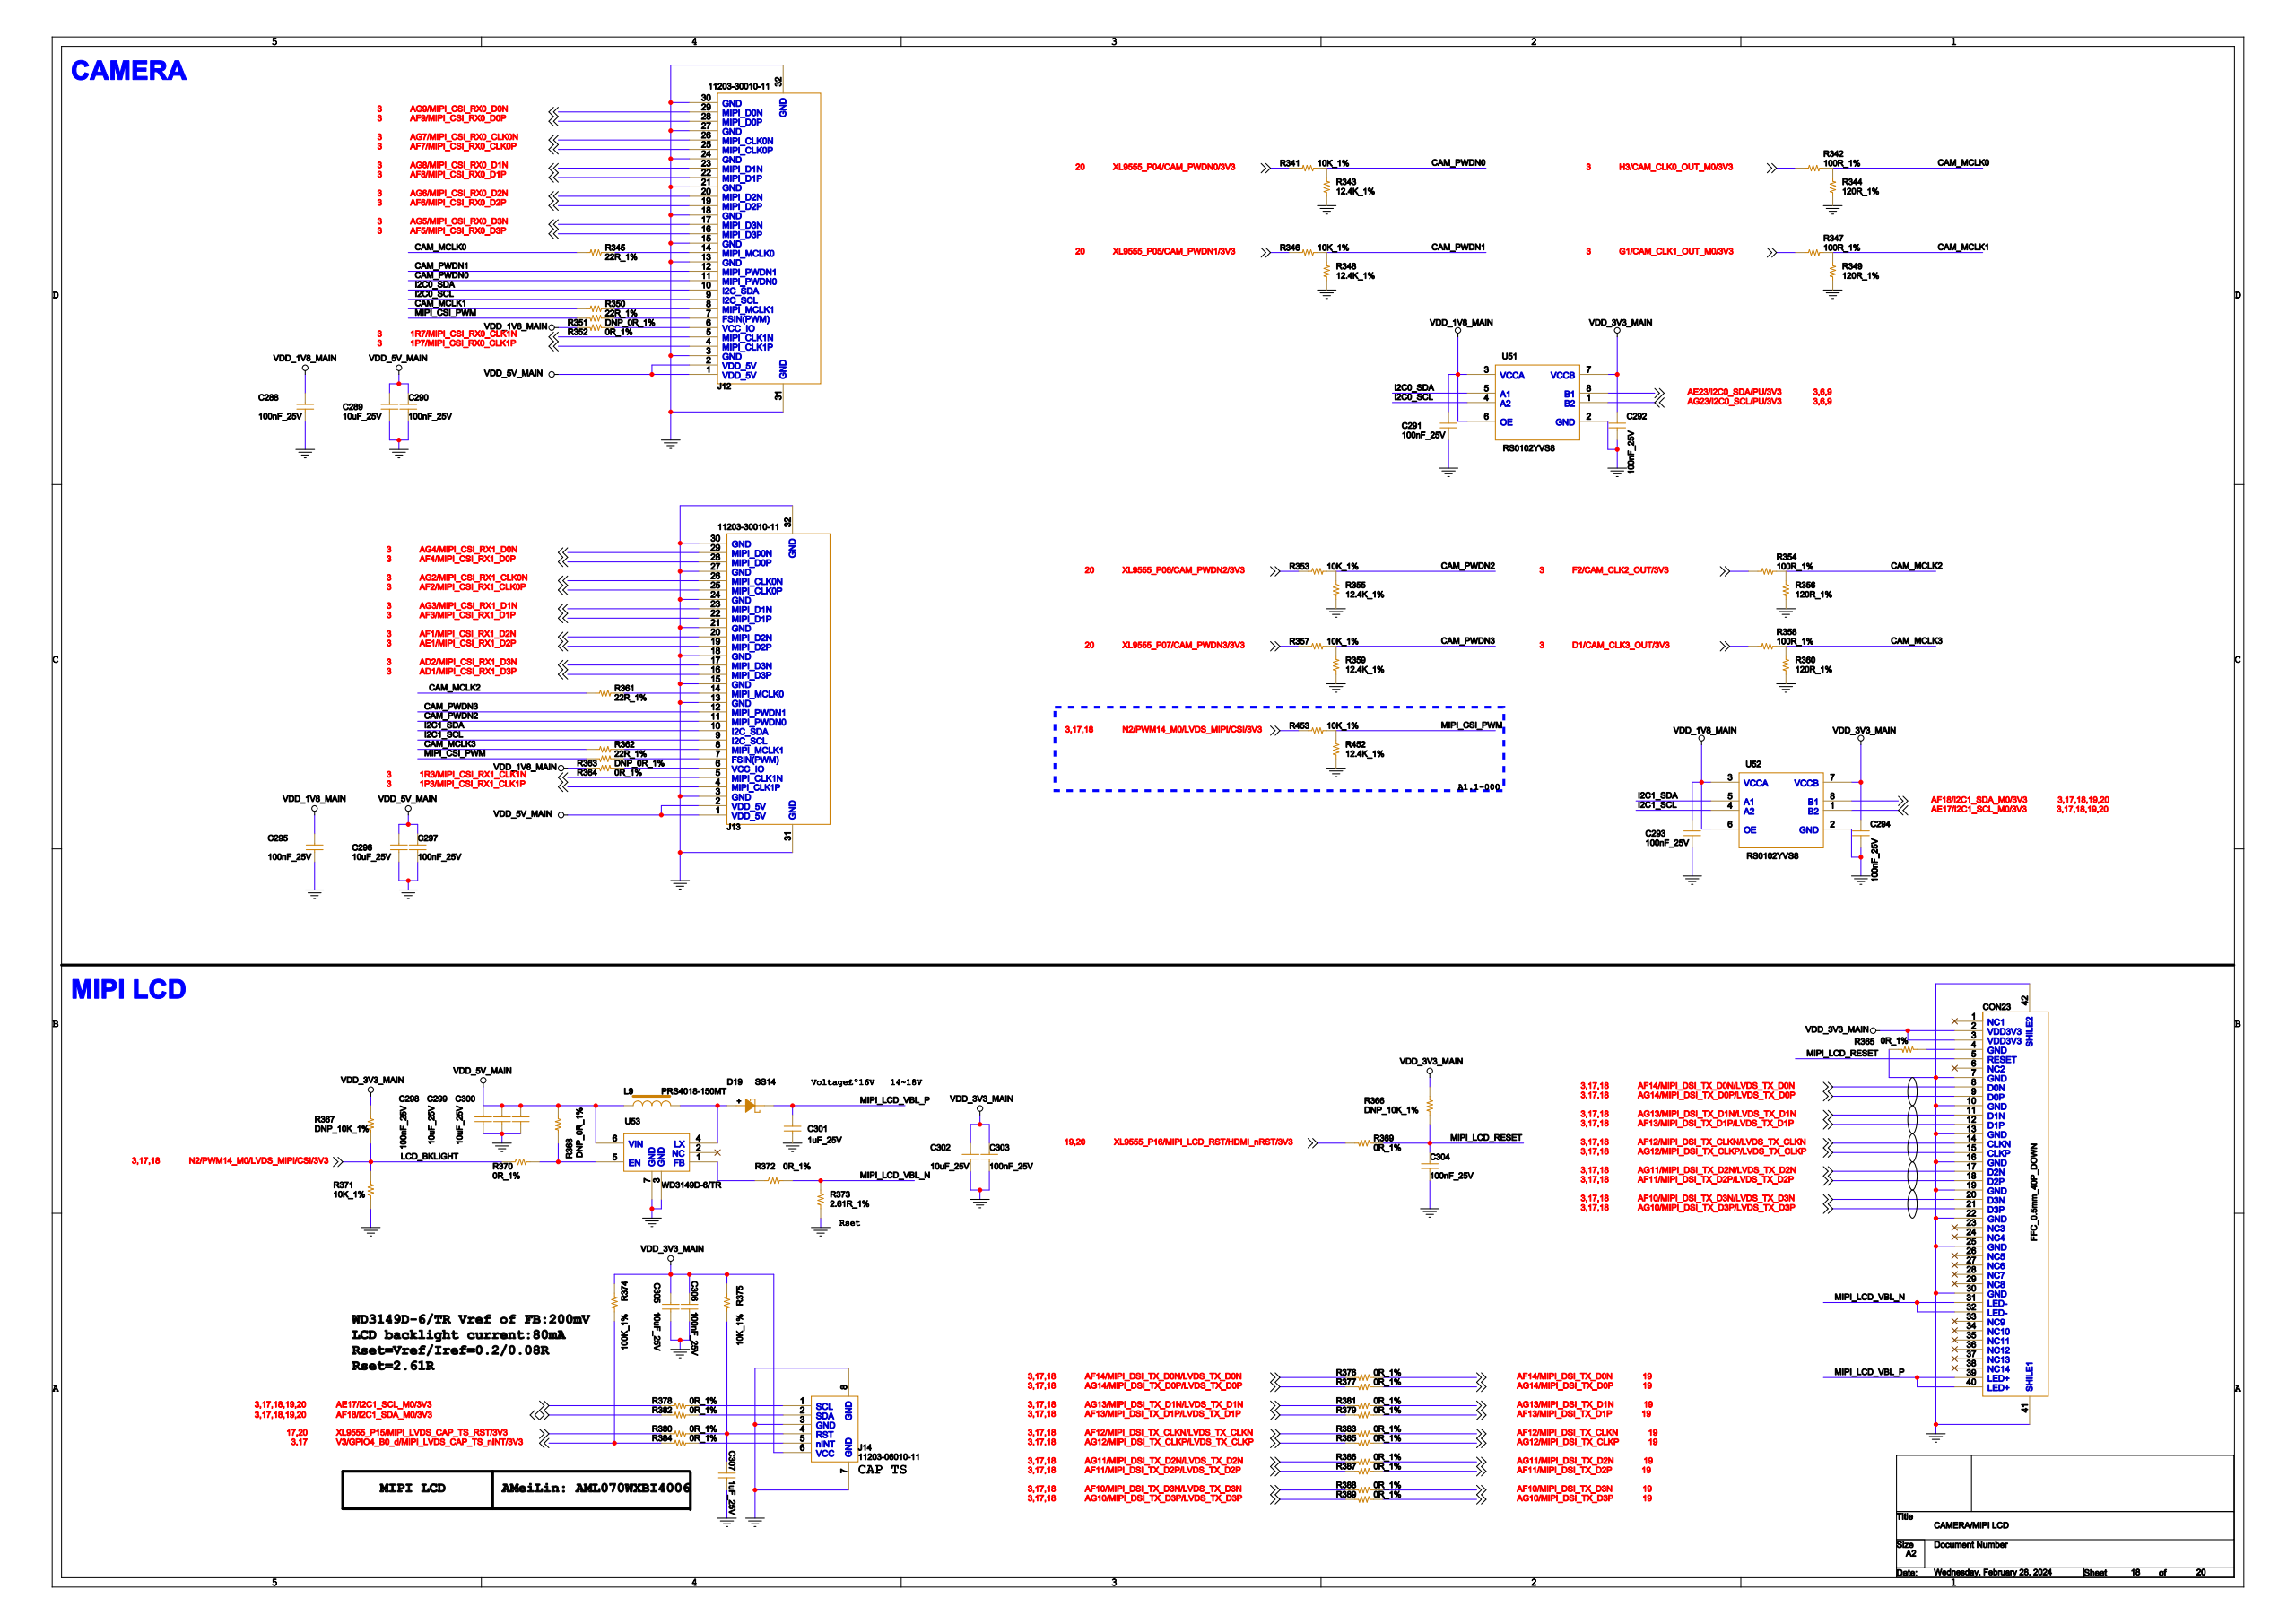Circuit board | Cadence Allegro | 1024 parts | 682 nets | one sheet of the schematic
Parts on this sheet (reference | value | footprint):
C288 | 100nF_25V | C0402
C289 | 10uF_25V | C0603
C290 | 100nF_25V | C0402
C291 | 100nF_25V | C0402
C292 | 100nF_25V | C0402
C293 | 100nF_25V | C0402
C294 | 100nF_25V | C0402
C295 | 100nF_25V | C0402
C296 | 10uF_25V | C0603
C297 | 100nF_25V | C0402
C298 | 100nF_25V | C0402
C299 | 10uF_25V | C0603
C300 | 10uF_25V | C0603
C301 | 1uF_25V | C0603
C302 | 10uF_25V | C0603
C303 | 100nF_25V | C0402
C304 | 100nF_25V | C0402
C305 | 10uF_25V | C0603
C306 | 100nF_25V | C0402
C307 | 1uF_25V | C0603
CON23 | FFC_0.5mm_40P_DOWN | CON_FFC_0D5_40P
D19 | SS14 | SMA
J12 | 11203-30010-11 | CON_FFC_0D5_30P
J13 | 11203-30010-11 | CON_FFC_0D5_30P
J14 | 11203-06010-11 | CON_FFC_0D5_6P
L9 | PRS4018-150MT | L_L4D5XW4D0_H3D2
R341 | 10K_1% | R0402
R342 | 100R_1% | R0603
R343 | 12.4K_1% | R0402
R344 | 120R_1% | R0603
R345 | 22R_1% | R0402
R346 | 10K_1% | R0402
R347 | 100R_1% | R0603
R348 | 12.4K_1% | R0402
R349 | 120R_1% | R0603
R350 | 22R_1% | R0402
R351 | DNP_0R_1% | R0402
R352 | 0R_1% | R0402
R353 | 10K_1% | R0402
R354 | 100R_1% | R0603
R355 | 12.4K_1% | R0402
R356 | 120R_1% | R0603
R357 | 10K_1% | R0402
R358 | 100R_1% | R0603
R359 | 12.4K_1% | R0402
R360 | 120R_1% | R0603
R361 | 22R_1% | R0402
R362 | 22R_1% | R0402
R363 | DNP_0R_1% | R0402
R364 | 0R_1% | R0402
R365 | 0R_1% | R0402
R366 | DNP_10K_1% | R0402
R367 | DNP_10K_1% | R0402
R368 | DNP_0R_1% | R0402
R369 | 0R_1% | R0402
R370 | 0R_1% | R0402
R371 | 10K_1% | R0402
R372 | 0R_1% | R0402
R373 | 2.61R_1% | R0402
R374 | 100K_1% | R0402
R375 | 10K_1% | R0402
R376 | 0R_1% | R0402
R377 | 0R_1% | R0402
R378 | 0R_1% | R0402
R379 | 0R_1% | R0402
R380 | 0R_1% | R0402
R381 | 0R_1% | R0402
R382 | 0R_1% | R0402
R383 | 0R_1% | R0402
R384 | 0R_1% | R0402
R385 | 0R_1% | R0402
R386 | 0R_1% | R0402
R387 | 0R_1% | R0402
R388 | 0R_1% | R0402
R389 | 0R_1% | R0402
R452 | 12.4K_1% | R0402
R453 | 10K_1% | R0402
U51 | RS0102YVS8 | SOP8-20-91
U52 | RS0102YVS8 | SOP8-20-91
U53 | WD3149D-6/TR | DFN2X2-6L
Nets of these parts (net: part-pin ...):
GND: C288-2 C289-2 C290-2 C291-2 C292-2 C293-2 C294-2 C295-2 C296-2 C297-2 C298-2 C299-2 C300-2 C301-2 C302-2 C303-2 C304-2 C305-2 C306-2 C307-2 J14-3 J14-7 J14-8 R343-1 R344-1 R348-1 R349-1 R355-1 R356-1 R359-1 R360-1 R365-1 R371-1 R373-2 R452-1 U51-2 U52-2 U53-3 U53-7 CON23-7 CON23-10 CON23-13 CON23-16 CON23-19 CON23-22 CON23-25 CON23-30 CON23-41 CON23-42 J12-3 J12-13 J12-15 J12-18 J12-21 J12-24 J12-27 J12-30 J12-31 J12-32 J13-3 J13-13 J13-15 J13-18 J13-21 J13-24 J13-27 J13-30 J13-31 J13-32
N21702476: R350-2 J12-8
CAM_PWDN1: R346-1 R348-2 J12-12
N21892162: R351-1 J12-7
I2C0_SCL: U51-4 J12-9
I2C0_SDA: U51-5 J12-10
AG7/MIPI_CSI_RX0_CLK0N: J12-26
AF7/MIPI_CSI_RX0_CLK0P: J12-25
1R7/MIPI_CSI_RX0_CLK1N: J12-5
1P7/MIPI_CSI_RX0_CLK1P: J12-4
AG9/MIPI_CSI_RX0_D0N: J12-29
AF9/MIPI_CSI_RX0_D0P: J12-28
AG8/MIPI_CSI_RX0_D1N: J12-23
AF8/MIPI_CSI_RX0_D1P: J12-22
AG6/MIPI_CSI_RX0_D2N: J12-20
AF6/MIPI_CSI_RX0_D2P: J12-19
AG5/MIPI_CSI_RX0_D3N: J12-17
AF5/MIPI_CSI_RX0_D3P: J12-16
N21690789: R345-2 J12-14
CAM_PWDN0: R341-1 R343-2 J12-11
N21690737: R352-1 J12-6
VDD_5V_MAIN: C289-1 C290-1 C296-1 C297-1 C298-1 C299-1 C300-1 L9-1 R368-2 U53-6 J12-1 J12-2 J13-1 J13-2
N21777437: R362-2 J13-8
CAM_PWDN3: R357-1 R359-2 J13-12
N21892001: R363-1 J13-7
I2C1_SCL: U52-4 J13-9
I2C1_SDA: U52-5 J13-10
AG2/MIPI_CSI_RX1_CLK0N: J13-26
AF2/MIPI_CSI_RX1_CLK0P: J13-25
1R3/MIPI_CSI_RX1_CLK1N: J13-5
1P3/MIPI_CSI_RX1_CLK1P: J13-4
AG4/MIPI_CSI_RX1_D0N: J13-29
AF4/MIPI_CSI_RX1_D0P: J13-28
AG3/MIPI_CSI_RX1_D1N: J13-23
AF3/MIPI_CSI_RX1_D1P: J13-22
AF1/MIPI_CSI_RX1_D2N: J13-20
AE1/MIPI_CSI_RX1_D2P: J13-19
AD2/MIPI_CSI_RX1_D3N: J13-17
AD1/MIPI_CSI_RX1_D3P: J13-16
N21697017: R361-2 J13-14
CAM_PWDN2: R353-1 R355-2 J13-11
N21696965: R364-1 J13-6
VDD_1V8_MAIN: C288-1 C291-1 C293-1 C295-1 R352-2 R364-2 U51-3 U51-6 U52-3 U52-6
AF10/MIPI_DSI_TX_D3N/LVDS_TX_D3: R388-1 CON23-20
AG10/MIPI_DSI_TX_D3P/LVDS_TX_D3: R389-1 CON23-21
AF12/MIPI_DSI_TX_CLKN/LVDS_TX_C: R383-1 CON23-14
AG12/MIPI_DSI_TX_CLKP/LVDS_TX_C: R385-1 CON23-15
AG11/MIPI_DSI_TX_D2N/LVDS_TX_D2: R386-1 CON23-17
AF11/MIPI_DSI_TX_D2P/LVDS_TX_D2: R387-1 CON23-18
AG13/MIPI_DSI_TX_D1N/LVDS_TX_D1: R381-1 CON23-11
AF13/MIPI_DSI_TX_D1P/LVDS_TX_D1: R379-1 CON23-12
AF14/MIPI_DSI_TX_D0N/LVDS_TX_D0: R376-1 CON23-8
AG14/MIPI_DSI_TX_D0P/LVDS_TX_D0: R377-1 CON23-9
VDD_3V3_MAIN: C292-1 C294-1 C302-1 C303-1 C305-1 C306-1 J14-6 R366-1 R367-2 R374-1 R375-1 U51-7 U52-7 CON23-2 CON23-3
AF18/I2C1_SDA_M0/3V3: R382-1 U52-8
AE17/I2C1_SCL_M0/3V3: R378-1 U52-1
AE23/I2C0_SDA/PU/3V3: U51-8
AG23/I2C0_SCL/PU/3V3: U51-1
V3/GPIO4_B0_D/MIPI_LVDS_CAP_TS_: R374-2 R384-1
N2/PWM14_M0/LVDS_MIPI/CSI/3V3: R367-1 R370-1 R371-2 R453-2
H3/CAM_CLK0_OUT_M0/3V3: R342-2
F2/CAM_CLK2_OUT/3V3: R354-2
G1/CAM_CLK1_OUT_M0/3V3: R347-2
D1/CAM_CLK3_OUT/3V3: R358-2
XL9555_P15/MIPI_LVDS_CAP_TS_RST: R380-1
N21631753: J14-5 R384-2
N21631711: C307-1 J14-4 R375-2 R380-2
N21631707: J14-1 R378-2
N21631705: J14-2 R382-2
MIPI_CSI_PWM: R351-2 R363-2 R452-2 R453-1
N21631565: R368-1 R370-2 U53-5
N21631446: R372-1 U53-1
N21631541: D19-1 L9-2 U53-4
AF12/MIPI_DSI_TX_CLKN: R383-2
AG12/MIPI_DSI_TX_CLKP: R385-2
AF14/MIPI_DSI_TX_D0N: R376-2
AG14/MIPI_DSI_TX_D0P: R377-2
AG13/MIPI_DSI_TX_D1N: R381-2
AF13/MIPI_DSI_TX_D1P: R379-2
AG11/MIPI_DSI_TX_D2N: R386-2
AF11/MIPI_DSI_TX_D2P: R387-2
AF10/MIPI_DSI_TX_D3N: R388-2
AG10/MIPI_DSI_TX_D3P: R389-2
XL9555_P04/CAM_PWDN0/3V3: R341-2
XL9555_P05/CAM_PWDN1/3V3: R346-2
XL9555_P06/CAM_PWDN2/3V3: R353-2
XL9555_P07/CAM_PWDN3/3V3: R357-2
XL9555_P16/MIPI_LCD_RST/HDMI_NR: R369-1
CAM_MCLK0: R342-1 R344-2 R345-1
CAM_MCLK1: R347-1 R349-2 R350-1
CAM_MCLK2: R354-1 R356-2 R361-1
CAM_MCLK3: R358-1 R360-2 R362-1
N21631371: R365-2 CON23-4
MIPI_LCD_RESET: C304-1 R366-2 R369-2 CON23-5
MIPI_LCD_VBL_N: R372-2 R373-1 CON23-31 CON23-32
MIPI_LCD_VBL_P: C301-1 D19-2 CON23-39 CON23-40